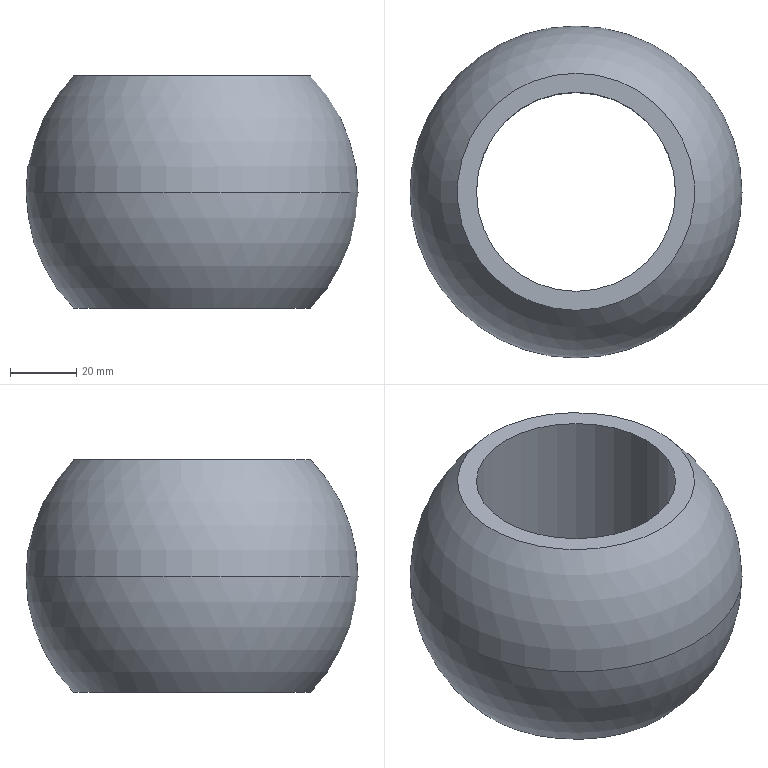Part | SolidWorks | features ICE 2, Revolution 1 | 1 solid | 6 faces | box 100 x 100 x 70 mm | volume 262061 mm3 | sphere 2 | cylinder 2 | plane 2 | commonest cylinder face diameters 60 x2
STEP:
#1=CARTESIAN_POINT('',(0.,35.707,-35.));
#2=VERTEX_POINT('',#1);
#3=CARTESIAN_POINT('',(0.,-35.707,-35.));
#4=VERTEX_POINT('',#3);
#5=CARTESIAN_POINT('',(0.,0.,-35.));
#6=DIRECTION('',(0.,0.,-1.));
#7=DIRECTION('',(0.,1.,0.));
#8=AXIS2_PLACEMENT_3D('',#5,#6,#7);
#9=CIRCLE('',#8,35.707);
#10=EDGE_CURVE('',#2,#4,#9,.T.);
#11=ORIENTED_EDGE('',*,*,#10,.F.);
#12=CARTESIAN_POINT('',(0.,0.,-35.));
#13=DIRECTION('',(0.,0.,-1.));
#14=DIRECTION('',(0.,1.,0.));
#15=AXIS2_PLACEMENT_3D('',#12,#13,#14);
#16=CIRCLE('',#15,35.707);
#17=EDGE_CURVE('',#4,#2,#16,.T.);
#18=ORIENTED_EDGE('',*,*,#17,.F.);
#19=EDGE_LOOP('',(#11,#18));
#20=FACE_BOUND('',#19,.T.);
#21=CARTESIAN_POINT('',(0.,-50.,0.));
#22=VERTEX_POINT('',#21);
#23=CARTESIAN_POINT('',(0.,50.,0.));
#24=VERTEX_POINT('',#23);
#25=CARTESIAN_POINT('',(0.,0.,0.));
#26=DIRECTION('',(0.,0.,1.));
#27=DIRECTION('',(1.,0.,0.));
#28=AXIS2_PLACEMENT_3D('',#25,#26,#27);
#29=CIRCLE('',#28,50.);
#30=EDGE_CURVE('',#22,#24,#29,.T.);
#31=ORIENTED_EDGE('',*,*,#30,.F.);
#32=CARTESIAN_POINT('',(0.,0.,0.));
#33=DIRECTION('',(0.,0.,-1.));
#34=DIRECTION('',(-1.,0.,0.));
#35=AXIS2_PLACEMENT_3D('',#32,#33,#34);
#36=CIRCLE('',#35,50.);
#37=EDGE_CURVE('',#22,#24,#36,.T.);
#38=ORIENTED_EDGE('',*,*,#37,.T.);
#39=EDGE_LOOP('',(#31,#38));
#40=FACE_OUTER_BOUND('',#39,.T.);
#41=CARTESIAN_POINT('',(0.,0.,0.));
#42=DIRECTION('',(0.,0.,-1.));
#43=DIRECTION('',(1.,0.,0.));
#44=AXIS2_PLACEMENT_3D('',#41,#42,#43);
#45=SPHERICAL_SURFACE('',#44,50.);
#46=ADVANCED_FACE('',(#20,#40),#45,.T.);
#47=CARTESIAN_POINT('',(-30.,0.,-35.));
#48=VERTEX_POINT('',#47);
#49=CARTESIAN_POINT('',(30.,0.,-35.));
#50=VERTEX_POINT('',#49);
#51=CARTESIAN_POINT('',(0.,0.,-35.));
#52=DIRECTION('',(0.,0.,1.));
#53=DIRECTION('',(0.,1.,0.));
#54=AXIS2_PLACEMENT_3D('',#51,#52,#53);
#55=CIRCLE('',#54,30.);
#56=EDGE_CURVE('',#48,#50,#55,.T.);
#57=ORIENTED_EDGE('',*,*,#56,.F.);
#58=CARTESIAN_POINT('',(-30.,0.,35.));
#59=VERTEX_POINT('',#58);
#60=CARTESIAN_POINT('',(-30.,0.,-50.));
#61=DIRECTION('',(0.,0.,1.));
#62=VECTOR('',#61,1000.);
#63=LINE('',#60,#62);
#64=EDGE_CURVE('',#48,#59,#63,.T.);
#65=ORIENTED_EDGE('',*,*,#64,.T.);
#66=CARTESIAN_POINT('',(30.,0.,35.));
#67=VERTEX_POINT('',#66);
#68=CARTESIAN_POINT('',(0.,0.,35.));
#69=DIRECTION('',(0.,0.,-1.));
#70=DIRECTION('',(0.,-1.,0.));
#71=AXIS2_PLACEMENT_3D('',#68,#69,#70);
#72=CIRCLE('',#71,30.);
#73=EDGE_CURVE('',#67,#59,#72,.T.);
#74=ORIENTED_EDGE('',*,*,#73,.F.);
#75=CARTESIAN_POINT('',(30.,0.,-50.));
#76=DIRECTION('',(0.,0.,1.));
#77=VECTOR('',#76,1000.);
#78=LINE('',#75,#77);
#79=EDGE_CURVE('',#50,#67,#78,.T.);
#80=ORIENTED_EDGE('',*,*,#79,.F.);
#81=EDGE_LOOP('',(#57,#65,#74,#80));
#82=FACE_OUTER_BOUND('',#81,.T.);
#83=CARTESIAN_POINT('',(0.,0.,-50.));
#84=DIRECTION('',(0.,0.,1.));
#85=DIRECTION('',(1.,0.,0.));
#86=AXIS2_PLACEMENT_3D('',#83,#84,#85);
#87=CYLINDRICAL_SURFACE('',#86,30.);
#88=ADVANCED_FACE('',(#82),#87,.F.);
#89=ORIENTED_EDGE('',*,*,#64,.F.);
#90=CARTESIAN_POINT('',(0.,0.,-35.));
#91=DIRECTION('',(0.,0.,1.));
#92=DIRECTION('',(0.,1.,0.));
#93=AXIS2_PLACEMENT_3D('',#90,#91,#92);
#94=CIRCLE('',#93,30.);
#95=EDGE_CURVE('',#50,#48,#94,.T.);
#96=ORIENTED_EDGE('',*,*,#95,.F.);
#97=ORIENTED_EDGE('',*,*,#79,.T.);
#98=CARTESIAN_POINT('',(0.,0.,35.));
#99=DIRECTION('',(0.,0.,-1.));
#100=DIRECTION('',(0.,-1.,0.));
#101=AXIS2_PLACEMENT_3D('',#98,#99,#100);
#102=CIRCLE('',#101,30.);
#103=EDGE_CURVE('',#59,#67,#102,.T.);
#104=ORIENTED_EDGE('',*,*,#103,.F.);
#105=EDGE_LOOP('',(#89,#96,#97,#104));
#106=FACE_OUTER_BOUND('',#105,.T.);
#107=CARTESIAN_POINT('',(0.,0.,-50.));
#108=DIRECTION('',(0.,0.,1.));
#109=DIRECTION('',(1.,0.,0.));
#110=AXIS2_PLACEMENT_3D('',#107,#108,#109);
#111=CYLINDRICAL_SURFACE('',#110,30.);
#112=ADVANCED_FACE('',(#106),#111,.F.);
#113=ORIENTED_EDGE('',*,*,#73,.T.);
#114=ORIENTED_EDGE('',*,*,#103,.T.);
#115=EDGE_LOOP('',(#113,#114));
#116=FACE_BOUND('',#115,.T.);
#117=CARTESIAN_POINT('',(0.,-35.707,35.));
#118=VERTEX_POINT('',#117);
#119=CARTESIAN_POINT('',(0.,35.707,35.));
#120=VERTEX_POINT('',#119);
#121=CARTESIAN_POINT('',(0.,0.,35.));
#122=DIRECTION('',(0.,0.,1.));
#123=DIRECTION('',(0.,-1.,0.));
#124=AXIS2_PLACEMENT_3D('',#121,#122,#123);
#125=CIRCLE('',#124,35.707);
#126=EDGE_CURVE('',#118,#120,#125,.T.);
#127=ORIENTED_EDGE('',*,*,#126,.T.);
#128=CARTESIAN_POINT('',(0.,0.,35.));
#129=DIRECTION('',(0.,0.,1.));
#130=DIRECTION('',(0.,-1.,0.));
#131=AXIS2_PLACEMENT_3D('',#128,#129,#130);
#132=CIRCLE('',#131,35.707);
#133=EDGE_CURVE('',#120,#118,#132,.T.);
#134=ORIENTED_EDGE('',*,*,#133,.T.);
#135=EDGE_LOOP('',(#127,#134));
#136=FACE_OUTER_BOUND('',#135,.T.);
#137=CARTESIAN_POINT('',(-50.,60.,35.));
#138=DIRECTION('',(0.,0.,1.));
#139=DIRECTION('',(0.,-1.,0.));
#140=AXIS2_PLACEMENT_3D('',#137,#138,#139);
#141=PLANE('',#140);
#142=ADVANCED_FACE('',(#116,#136),#141,.T.);
#143=ORIENTED_EDGE('',*,*,#95,.T.);
#144=ORIENTED_EDGE('',*,*,#56,.T.);
#145=EDGE_LOOP('',(#143,#144));
#146=FACE_BOUND('',#145,.T.);
#147=ORIENTED_EDGE('',*,*,#10,.T.);
#148=ORIENTED_EDGE('',*,*,#17,.T.);
#149=EDGE_LOOP('',(#147,#148));
#150=FACE_OUTER_BOUND('',#149,.T.);
#151=CARTESIAN_POINT('',(-50.,60.,-35.));
#152=DIRECTION('',(0.,0.,-1.));
#153=DIRECTION('',(0.,1.,0.));
#154=AXIS2_PLACEMENT_3D('',#151,#152,#153);
#155=PLANE('',#154);
#156=ADVANCED_FACE('',(#146,#150),#155,.T.);
#157=ORIENTED_EDGE('',*,*,#37,.F.);
#158=ORIENTED_EDGE('',*,*,#30,.T.);
#159=EDGE_LOOP('',(#157,#158));
#160=FACE_OUTER_BOUND('',#159,.T.);
#161=ORIENTED_EDGE('',*,*,#126,.F.);
#162=ORIENTED_EDGE('',*,*,#133,.F.);
#163=EDGE_LOOP('',(#161,#162));
#164=FACE_BOUND('',#163,.T.);
#165=CARTESIAN_POINT('',(0.,0.,0.));
#166=DIRECTION('',(0.,0.,-1.));
#167=DIRECTION('',(1.,0.,0.));
#168=AXIS2_PLACEMENT_3D('',#165,#166,#167);
#169=SPHERICAL_SURFACE('',#168,50.);
#170=ADVANCED_FACE('',(#160,#164),#169,.T.);
#171=CLOSED_SHELL('',(#46,#88,#112,#142,#156,#170));
#172=MANIFOLD_SOLID_BREP('',#171);
#173=CARTESIAN_POINT('',(0.,0.,0.));
#174=DIRECTION('',(0.,0.,1.));
#175=DIRECTION('',(1.,0.,0.));
#176=AXIS2_PLACEMENT_3D('',#173,#174,#175);
#177=(LENGTH_UNIT()NAMED_UNIT(*)SI_UNIT(.MILLI.,.METRE.));
#178=UNCERTAINTY_MEASURE_WITH_UNIT(LENGTH_MEASURE(0.00001),#177,'','');
#179=(NAMED_UNIT(*)PLANE_ANGLE_UNIT()SI_UNIT($,.RADIAN.));
#180=(NAMED_UNIT(*)SI_UNIT($,.STERADIAN.)SOLID_ANGLE_UNIT());
#181=(GEOMETRIC_REPRESENTATION_CONTEXT(3)GLOBAL_UNCERTAINTY_ASSIGNED_CONTEXT((#178))GLOBAL_UNIT_ASSIGNED_CONTEXT((#177,#179,#180))REPRESENTATION_CONTEXT('',''));
#182=ADVANCED_BREP_SHAPE_REPRESENTATION('',(#172,#176),#181);